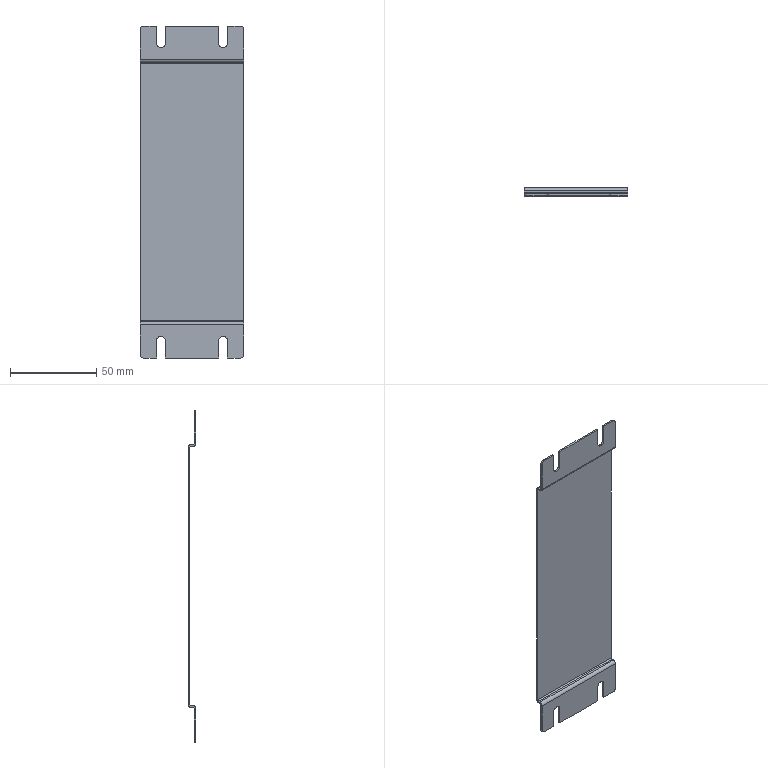Part | STEP file | Card reader Clamp plate | 1 solid | 60 faces | box 60 x 4.5 x 192 mm | volume 11570 mm3 | plane 42 | cylinder 18 | commonest cylinder face diameters 5 x6 1.473 x4 3.473 x4 4 x4